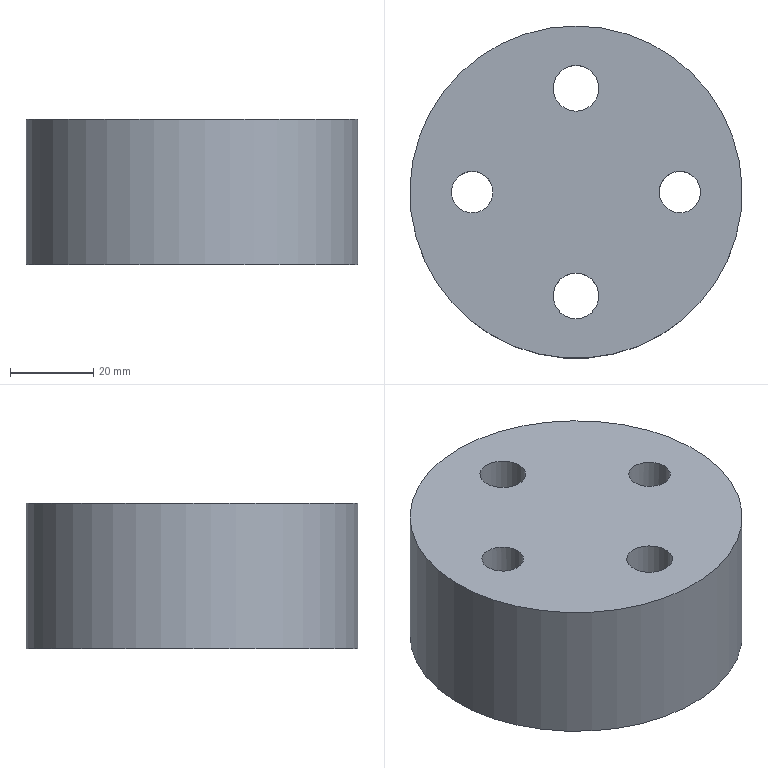Part | NX | features solid 2 | 1 solid | 14 faces | box 80 x 80 x 35 mm | volume 136848 mm3 | cylinder 8 | plane 5 | cone 1 | commonest cylinder face diameters 10 x2 11 x2 17 x2 5 x1 80 x1
STEP:
#1=CARTESIAN_POINT('',(1230.,-115.,-10.));
#2=VERTEX_POINT('',#1);
#3=CARTESIAN_POINT('',(1230.,-155.,-10.));
#4=DIRECTION('',(0.,0.,1.));
#5=DIRECTION('',(0.,1.,0.));
#6=AXIS2_PLACEMENT_3D('',#3,#4,#5);
#7=CIRCLE('',#6,40.);
#8=EDGE_CURVE('',#2,#2,#7,.T.);
#9=ORIENTED_EDGE('',*,*,#8,.F.);
#10=EDGE_LOOP('',(#9));
#11=FACE_BOUND('',#10,.T.);
#12=CARTESIAN_POINT('',(1230.,-121.225,-10.));
#13=VERTEX_POINT('',#12);
#14=CARTESIAN_POINT('',(1230.,-155.,-10.));
#15=DIRECTION('',(0.,0.,1.));
#16=DIRECTION('',(0.,1.,0.));
#17=AXIS2_PLACEMENT_3D('',#14,#15,#16);
#18=CIRCLE('',#17,33.775);
#19=EDGE_CURVE('',#13,#13,#18,.F.);
#20=ORIENTED_EDGE('',*,*,#19,.F.);
#21=EDGE_LOOP('',(#20));
#22=FACE_BOUND('',#21,.T.);
#23=CARTESIAN_POINT('',(1230.,-155.,-10.));
#24=DIRECTION('',(0.,0.,-1.));
#25=DIRECTION('',(0.,1.,0.));
#26=AXIS2_PLACEMENT_3D('',#23,#24,#25);
#27=PLANE('',#26);
#28=ADVANCED_FACE('',(#11,#22),#27,.T.);
#29=CARTESIAN_POINT('',(1230.,-171.5,15.));
#30=VERTEX_POINT('',#29);
#31=CARTESIAN_POINT('',(1230.,-180.,15.));
#32=DIRECTION('',(0.,0.,1.));
#33=DIRECTION('',(0.,1.,0.));
#34=AXIS2_PLACEMENT_3D('',#31,#32,#33);
#35=CIRCLE('',#34,8.5);
#36=EDGE_CURVE('',#30,#30,#35,.T.);
#37=ORIENTED_EDGE('',*,*,#36,.T.);
#38=EDGE_LOOP('',(#37));
#39=FACE_BOUND('',#38,.T.);
#40=CARTESIAN_POINT('',(1232.133,-171.772,-0.2613));
#41=VERTEX_POINT('',#40);
#42=CARTESIAN_POINT('',(1235.334,-173.116,-1.388));
#43=CARTESIAN_POINT('',(1232.24,-171.537,-0.06708));
#44=CARTESIAN_POINT('',(1228.503,-171.368,0.0881));
#45=CARTESIAN_POINT('',(1225.219,-172.711,-1.068));
#46=CARTESIAN_POINT('',(1222.909,-174.976,-2.736));
#47=CARTESIAN_POINT('',(1221.135,-178.794,-5.162));
#48=CARTESIAN_POINT('',(1221.604,-183.266,-7.482));
#49=CARTESIAN_POINT('',(1224.537,-186.821,-9.112));
#50=CARTESIAN_POINT('',(1227.755,-188.463,-9.826));
#51=CARTESIAN_POINT('',(1231.445,-188.641,-9.902));
#52=CARTESIAN_POINT('',(1235.993,-186.822,-9.118));
#53=CARTESIAN_POINT('',(1238.545,-182.748,-7.247));
#54=CARTESIAN_POINT('',(1238.556,-178.475,-4.925));
#55=CARTESIAN_POINT('',(1237.446,-175.519,-3.102));
#56=CARTESIAN_POINT('',(1235.334,-173.116,-1.388));
#57=CARTESIAN_POINT('',(1232.24,-171.537,-0.06708));
#58=CARTESIAN_POINT('',(1228.503,-171.368,0.0881));
#59=B_SPLINE_CURVE_WITH_KNOTS('',3,(#42,#43,#44,#45,#46,#47,#48,#49,#50,#51,#52,#53,#54,#55,#56,#57,#58),.UNSPECIFIED.,.T.,.F.,(1,1,1,1,1,1,1,1,1,1,1,1,1,1,1,1,1,1,1,1,1),(-0.01077,-0.007179,-0.00359,0.,0.00359,0.007179,0.01077,0.01436,0.02154,0.02513,0.02872,0.03231,0.0359,0.04307,0.04666,0.05025,0.05384,0.05743,0.06102,0.06461,0.0682),.UNSPECIFIED.);
#60=EDGE_CURVE('',#41,#41,#59,.T.);
#61=ORIENTED_EDGE('',*,*,#60,.F.);
#62=EDGE_LOOP('',(#61));
#63=FACE_BOUND('',#62,.T.);
#64=CARTESIAN_POINT('',(1230.,-180.,-10.));
#65=DIRECTION('',(0.,0.,1.));
#66=DIRECTION('',(0.,-1.,0.));
#67=AXIS2_PLACEMENT_3D('',#64,#65,#66);
#68=CYLINDRICAL_SURFACE('',#67,8.5);
#69=ADVANCED_FACE('',(#39,#63),#68,.F.);
#70=CARTESIAN_POINT('',(1230.,-121.5,15.));
#71=VERTEX_POINT('',#70);
#72=CARTESIAN_POINT('',(1230.,-130.,15.));
#73=DIRECTION('',(0.,0.,1.));
#74=DIRECTION('',(0.,1.,0.));
#75=AXIS2_PLACEMENT_3D('',#72,#73,#74);
#76=CIRCLE('',#75,8.5);
#77=EDGE_CURVE('',#71,#71,#76,.T.);
#78=ORIENTED_EDGE('',*,*,#77,.T.);
#79=EDGE_LOOP('',(#78));
#80=FACE_BOUND('',#79,.T.);
#81=CARTESIAN_POINT('',(1232.133,-138.228,-0.2613));
#82=VERTEX_POINT('',#81);
#83=CARTESIAN_POINT('',(1228.487,-138.633,0.08799));
#84=CARTESIAN_POINT('',(1232.248,-138.46,-0.06903));
#85=CARTESIAN_POINT('',(1235.319,-136.894,-1.38));
#86=CARTESIAN_POINT('',(1237.448,-134.481,-3.102));
#87=CARTESIAN_POINT('',(1238.554,-131.529,-4.923));
#88=CARTESIAN_POINT('',(1238.547,-127.268,-7.238));
#89=CARTESIAN_POINT('',(1236.016,-123.209,-9.105));
#90=CARTESIAN_POINT('',(1231.512,-121.372,-9.896));
#91=CARTESIAN_POINT('',(1227.809,-121.519,-9.834));
#92=CARTESIAN_POINT('',(1224.566,-123.154,-9.123));
#93=CARTESIAN_POINT('',(1222.35,-125.818,-7.901));
#94=CARTESIAN_POINT('',(1221.36,-128.972,-6.327));
#95=CARTESIAN_POINT('',(1221.58,-132.155,-4.557));
#96=CARTESIAN_POINT('',(1222.906,-135.021,-2.739));
#97=CARTESIAN_POINT('',(1225.207,-137.28,-1.075));
#98=CARTESIAN_POINT('',(1228.487,-138.633,0.08799));
#99=CARTESIAN_POINT('',(1232.248,-138.46,-0.06903));
#100=CARTESIAN_POINT('',(1235.319,-136.894,-1.38));
#101=B_SPLINE_CURVE_WITH_KNOTS('',3,(#83,#84,#85,#86,#87,#88,#89,#90,#91,#92,#93,#94,#95,#96,#97,#98,#99,#100),.UNSPECIFIED.,.T.,.F.,(1,1,1,1,1,1,1,1,1,1,1,1,1,1,1,1,1,1,1,1,1,1),(-0.01073,-0.007156,-0.003578,0.,0.003578,0.007156,0.01073,0.01431,0.02147,0.02505,0.02862,0.0322,0.03578,0.03936,0.04294,0.04651,0.05009,0.05367,0.05725,0.06083,0.0644,0.06798),.UNSPECIFIED.);
#102=EDGE_CURVE('',#82,#82,#101,.T.);
#103=ORIENTED_EDGE('',*,*,#102,.F.);
#104=EDGE_LOOP('',(#103));
#105=FACE_BOUND('',#104,.T.);
#106=CARTESIAN_POINT('',(1230.,-130.,-10.));
#107=DIRECTION('',(0.,0.,1.));
#108=DIRECTION('',(0.,-1.,0.));
#109=AXIS2_PLACEMENT_3D('',#106,#107,#108);
#110=CYLINDRICAL_SURFACE('',#109,8.5);
#111=ADVANCED_FACE('',(#80,#105),#110,.F.);
#112=CARTESIAN_POINT('',(1255.,-150.,25.));
#113=VERTEX_POINT('',#112);
#114=CARTESIAN_POINT('',(1255.,-155.,25.));
#115=DIRECTION('',(0.,0.,1.));
#116=DIRECTION('',(0.,1.,0.));
#117=AXIS2_PLACEMENT_3D('',#114,#115,#116);
#118=CIRCLE('',#117,5.);
#119=EDGE_CURVE('',#113,#113,#118,.T.);
#120=ORIENTED_EDGE('',*,*,#119,.T.);
#121=EDGE_LOOP('',(#120));
#122=FACE_BOUND('',#121,.T.);
#123=CARTESIAN_POINT('',(1255.794,-159.937,-5.662));
#124=VERTEX_POINT('',#123);
#125=CARTESIAN_POINT('',(1252.677,-159.733,-3.871));
#126=CARTESIAN_POINT('',(1255.826,-160.41,-5.731));
#127=CARTESIAN_POINT('',(1258.815,-158.719,-7.248));
#128=CARTESIAN_POINT('',(1260.021,-156.153,-7.831));
#129=CARTESIAN_POINT('',(1260.063,-153.241,-7.851));
#130=CARTESIAN_POINT('',(1257.855,-150.263,-6.789));
#131=CARTESIAN_POINT('',(1254.604,-149.757,-5.026));
#132=CARTESIAN_POINT('',(1252.298,-150.657,-3.614));
#133=CARTESIAN_POINT('',(1250.872,-151.956,-2.67));
#134=CARTESIAN_POINT('',(1249.984,-153.829,-2.036));
#135=CARTESIAN_POINT('',(1249.95,-156.028,-2.012));
#136=CARTESIAN_POINT('',(1250.8,-157.948,-2.619));
#137=CARTESIAN_POINT('',(1252.677,-159.733,-3.871));
#138=CARTESIAN_POINT('',(1255.826,-160.41,-5.731));
#139=CARTESIAN_POINT('',(1258.815,-158.719,-7.248));
#140=B_SPLINE_CURVE_WITH_KNOTS('',3,(#125,#126,#127,#128,#129,#130,#131,#132,#133,#134,#135,#136,#137,#138,#139),.UNSPECIFIED.,.T.,.F.,(1,1,1,1,1,1,1,1,1,1,1,1,1,1,1,1,1,1,1),(-0.008415,-0.006311,-0.004207,0.,0.004207,0.006311,0.008415,0.01262,0.01683,0.01893,0.02104,0.02314,0.02524,0.02735,0.02945,0.03366,0.03787,0.03997,0.04207),.UNSPECIFIED.);
#141=EDGE_CURVE('',#124,#124,#140,.T.);
#142=ORIENTED_EDGE('',*,*,#141,.F.);
#143=EDGE_LOOP('',(#142));
#144=FACE_BOUND('',#143,.T.);
#145=CARTESIAN_POINT('',(1255.,-155.,-10.));
#146=DIRECTION('',(0.,0.,1.));
#147=DIRECTION('',(0.,-1.,0.));
#148=AXIS2_PLACEMENT_3D('',#145,#146,#147);
#149=CYLINDRICAL_SURFACE('',#148,5.);
#150=ADVANCED_FACE('',(#122,#144),#149,.F.);
#151=CARTESIAN_POINT('',(1205.,-150.,25.));
#152=VERTEX_POINT('',#151);
#153=CARTESIAN_POINT('',(1205.,-155.,25.));
#154=DIRECTION('',(0.,0.,1.));
#155=DIRECTION('',(0.,1.,0.));
#156=AXIS2_PLACEMENT_3D('',#153,#154,#155);
#157=CIRCLE('',#156,5.);
#158=EDGE_CURVE('',#152,#152,#157,.T.);
#159=ORIENTED_EDGE('',*,*,#158,.T.);
#160=EDGE_LOOP('',(#159));
#161=FACE_BOUND('',#160,.T.);
#162=CARTESIAN_POINT('',(1209.151,-157.787,-2.644));
#163=VERTEX_POINT('',#162);
#164=CARTESIAN_POINT('',(1207.856,-159.244,-3.515));
#165=CARTESIAN_POINT('',(1209.247,-157.882,-2.587));
#166=CARTESIAN_POINT('',(1210.064,-155.948,-2.001));
#167=CARTESIAN_POINT('',(1210.,-153.762,-2.048));
#168=CARTESIAN_POINT('',(1209.081,-151.891,-2.702));
#169=CARTESIAN_POINT('',(1207.155,-150.194,-3.975));
#170=CARTESIAN_POINT('',(1204.,-149.617,-5.825));
#171=CARTESIAN_POINT('',(1201.052,-151.418,-7.313));
#172=CARTESIAN_POINT('',(1199.938,-154.037,-7.851));
#173=CARTESIAN_POINT('',(1200.012,-156.963,-7.815));
#174=CARTESIAN_POINT('',(1202.318,-159.83,-6.702));
#175=CARTESIAN_POINT('',(1205.581,-160.226,-4.919));
#176=CARTESIAN_POINT('',(1207.856,-159.244,-3.515));
#177=CARTESIAN_POINT('',(1209.247,-157.882,-2.587));
#178=CARTESIAN_POINT('',(1210.064,-155.948,-2.001));
#179=B_SPLINE_CURVE_WITH_KNOTS('',3,(#164,#165,#166,#167,#168,#169,#170,#171,#172,#173,#174,#175,#176,#177,#178),.UNSPECIFIED.,.T.,.F.,(1,1,1,1,1,1,1,1,1,1,1,1,1,1,1,1,1,1,1),(-0.008441,-0.004221,-0.00211,0.,0.00211,0.004221,0.006331,0.008441,0.01266,0.01688,0.01899,0.0211,0.02532,0.02954,0.03165,0.03376,0.03588,0.03799,0.0401),.UNSPECIFIED.);
#180=EDGE_CURVE('',#163,#163,#179,.T.);
#181=ORIENTED_EDGE('',*,*,#180,.F.);
#182=EDGE_LOOP('',(#181));
#183=FACE_BOUND('',#182,.T.);
#184=CARTESIAN_POINT('',(1205.,-155.,-10.));
#185=DIRECTION('',(0.,0.,1.));
#186=DIRECTION('',(0.,-1.,0.));
#187=AXIS2_PLACEMENT_3D('',#184,#185,#186);
#188=CYLINDRICAL_SURFACE('',#187,5.);
#189=ADVANCED_FACE('',(#161,#183),#188,.F.);
#190=ORIENTED_EDGE('',*,*,#119,.F.);
#191=EDGE_LOOP('',(#190));
#192=FACE_BOUND('',#191,.T.);
#193=CARTESIAN_POINT('',(1230.,-174.5,25.));
#194=VERTEX_POINT('',#193);
#195=CARTESIAN_POINT('',(1230.,-180.,25.));
#196=DIRECTION('',(0.,0.,1.));
#197=DIRECTION('',(0.,1.,0.));
#198=AXIS2_PLACEMENT_3D('',#195,#196,#197);
#199=CIRCLE('',#198,5.5);
#200=EDGE_CURVE('',#194,#194,#199,.T.);
#201=ORIENTED_EDGE('',*,*,#200,.F.);
#202=EDGE_LOOP('',(#201));
#203=FACE_BOUND('',#202,.T.);
#204=CARTESIAN_POINT('',(1230.,-115.,25.));
#205=VERTEX_POINT('',#204);
#206=CARTESIAN_POINT('',(1230.,-155.,25.));
#207=DIRECTION('',(0.,0.,1.));
#208=DIRECTION('',(0.,1.,0.));
#209=AXIS2_PLACEMENT_3D('',#206,#207,#208);
#210=CIRCLE('',#209,40.);
#211=EDGE_CURVE('',#205,#205,#210,.T.);
#212=ORIENTED_EDGE('',*,*,#211,.T.);
#213=EDGE_LOOP('',(#212));
#214=FACE_BOUND('',#213,.T.);
#215=CARTESIAN_POINT('',(1230.,-124.5,25.));
#216=VERTEX_POINT('',#215);
#217=CARTESIAN_POINT('',(1230.,-130.,25.));
#218=DIRECTION('',(0.,0.,1.));
#219=DIRECTION('',(0.,1.,0.));
#220=AXIS2_PLACEMENT_3D('',#217,#218,#219);
#221=CIRCLE('',#220,5.5);
#222=EDGE_CURVE('',#216,#216,#221,.T.);
#223=ORIENTED_EDGE('',*,*,#222,.F.);
#224=EDGE_LOOP('',(#223));
#225=FACE_BOUND('',#224,.T.);
#226=ORIENTED_EDGE('',*,*,#158,.F.);
#227=EDGE_LOOP('',(#226));
#228=FACE_BOUND('',#227,.T.);
#229=CARTESIAN_POINT('',(1230.,-155.,25.));
#230=DIRECTION('',(0.,0.,-1.));
#231=DIRECTION('',(0.,1.,0.));
#232=AXIS2_PLACEMENT_3D('',#229,#230,#231);
#233=PLANE('',#232);
#234=ADVANCED_FACE('',(#192,#203,#214,#225,#228),#233,.F.);
#235=ORIENTED_EDGE('',*,*,#77,.F.);
#236=EDGE_LOOP('',(#235));
#237=FACE_BOUND('',#236,.T.);
#238=CARTESIAN_POINT('',(1230.,-124.5,15.));
#239=VERTEX_POINT('',#238);
#240=CARTESIAN_POINT('',(1230.,-130.,15.));
#241=DIRECTION('',(0.,0.,1.));
#242=DIRECTION('',(0.,1.,0.));
#243=AXIS2_PLACEMENT_3D('',#240,#241,#242);
#244=CIRCLE('',#243,5.5);
#245=EDGE_CURVE('',#239,#239,#244,.T.);
#246=ORIENTED_EDGE('',*,*,#245,.T.);
#247=EDGE_LOOP('',(#246));
#248=FACE_BOUND('',#247,.T.);
#249=CARTESIAN_POINT('',(1230.,-130.,15.));
#250=DIRECTION('',(0.,0.,-1.));
#251=DIRECTION('',(0.,1.,0.));
#252=AXIS2_PLACEMENT_3D('',#249,#250,#251);
#253=PLANE('',#252);
#254=ADVANCED_FACE('',(#237,#248),#253,.T.);
#255=ORIENTED_EDGE('',*,*,#36,.F.);
#256=EDGE_LOOP('',(#255));
#257=FACE_BOUND('',#256,.T.);
#258=CARTESIAN_POINT('',(1230.,-174.5,15.));
#259=VERTEX_POINT('',#258);
#260=CARTESIAN_POINT('',(1230.,-180.,15.));
#261=DIRECTION('',(0.,0.,1.));
#262=DIRECTION('',(0.,1.,0.));
#263=AXIS2_PLACEMENT_3D('',#260,#261,#262);
#264=CIRCLE('',#263,5.5);
#265=EDGE_CURVE('',#259,#259,#264,.T.);
#266=ORIENTED_EDGE('',*,*,#265,.T.);
#267=EDGE_LOOP('',(#266));
#268=FACE_BOUND('',#267,.T.);
#269=CARTESIAN_POINT('',(1230.,-180.,15.));
#270=DIRECTION('',(0.,0.,-1.));
#271=DIRECTION('',(0.,1.,0.));
#272=AXIS2_PLACEMENT_3D('',#269,#270,#271);
#273=PLANE('',#272);
#274=ADVANCED_FACE('',(#257,#268),#273,.T.);
#275=ORIENTED_EDGE('',*,*,#8,.T.);
#276=EDGE_LOOP('',(#275));
#277=FACE_BOUND('',#276,.T.);
#278=ORIENTED_EDGE('',*,*,#211,.F.);
#279=EDGE_LOOP('',(#278));
#280=FACE_BOUND('',#279,.T.);
#281=CARTESIAN_POINT('',(1230.,-155.,-10.));
#282=DIRECTION('',(0.,0.,1.));
#283=DIRECTION('',(0.,-1.,0.));
#284=AXIS2_PLACEMENT_3D('',#281,#282,#283);
#285=CYLINDRICAL_SURFACE('',#284,40.);
#286=ADVANCED_FACE('',(#277,#280),#285,.T.);
#287=ORIENTED_EDGE('',*,*,#265,.F.);
#288=EDGE_LOOP('',(#287));
#289=FACE_BOUND('',#288,.T.);
#290=ORIENTED_EDGE('',*,*,#200,.T.);
#291=EDGE_LOOP('',(#290));
#292=FACE_BOUND('',#291,.T.);
#293=CARTESIAN_POINT('',(1230.,-180.,15.));
#294=DIRECTION('',(0.,0.,1.));
#295=DIRECTION('',(0.,-1.,0.));
#296=AXIS2_PLACEMENT_3D('',#293,#294,#295);
#297=CYLINDRICAL_SURFACE('',#296,5.5);
#298=ADVANCED_FACE('',(#289,#292),#297,.F.);
#299=ORIENTED_EDGE('',*,*,#245,.F.);
#300=EDGE_LOOP('',(#299));
#301=FACE_BOUND('',#300,.T.);
#302=ORIENTED_EDGE('',*,*,#222,.T.);
#303=EDGE_LOOP('',(#302));
#304=FACE_BOUND('',#303,.T.);
#305=CARTESIAN_POINT('',(1230.,-130.,15.));
#306=DIRECTION('',(0.,0.,1.));
#307=DIRECTION('',(0.,-1.,0.));
#308=AXIS2_PLACEMENT_3D('',#305,#306,#307);
#309=CYLINDRICAL_SURFACE('',#308,5.5);
#310=ADVANCED_FACE('',(#301,#304),#309,.F.);
#311=ORIENTED_EDGE('',*,*,#19,.T.);
#312=EDGE_LOOP('',(#311));
#313=FACE_BOUND('',#312,.T.);
#314=ORIENTED_EDGE('',*,*,#60,.T.);
#315=EDGE_LOOP('',(#314));
#316=FACE_BOUND('',#315,.T.);
#317=ORIENTED_EDGE('',*,*,#102,.T.);
#318=EDGE_LOOP('',(#317));
#319=FACE_BOUND('',#318,.T.);
#320=ORIENTED_EDGE('',*,*,#141,.T.);
#321=EDGE_LOOP('',(#320));
#322=FACE_BOUND('',#321,.T.);
#323=ORIENTED_EDGE('',*,*,#180,.T.);
#324=EDGE_LOOP('',(#323));
#325=FACE_BOUND('',#324,.T.);
#326=CARTESIAN_POINT('',(1230.,-152.5,8.057));
#327=VERTEX_POINT('',#326);
#328=CARTESIAN_POINT('',(1230.,-155.,8.057));
#329=DIRECTION('',(0.,0.,1.));
#330=DIRECTION('',(0.,1.,0.));
#331=AXIS2_PLACEMENT_3D('',#328,#329,#330);
#332=CIRCLE('',#331,2.5);
#333=EDGE_CURVE('',#327,#327,#332,.F.);
#334=ORIENTED_EDGE('',*,*,#333,.F.);
#335=EDGE_LOOP('',(#334));
#336=FACE_BOUND('',#335,.T.);
#337=CARTESIAN_POINT('',(1230.,-155.,-13.594));
#338=DIRECTION('',(0.,0.,-1.));
#339=DIRECTION('',(0.,1.,0.));
#340=AXIS2_PLACEMENT_3D('',#337,#338,#339);
#341=CONICAL_SURFACE('',#340,40.,1.047);
#342=ADVANCED_FACE('',(#313,#316,#319,#322,#325,#336),#341,.F.);
#343=CARTESIAN_POINT('',(1230.,-157.5,10.));
#344=VERTEX_POINT('',#343);
#345=CARTESIAN_POINT('',(1230.,-155.,10.));
#346=DIRECTION('',(0.,0.,-1.));
#347=DIRECTION('',(0.,-1.,0.));
#348=AXIS2_PLACEMENT_3D('',#345,#346,#347);
#349=CIRCLE('',#348,2.5);
#350=EDGE_CURVE('',#344,#344,#349,.T.);
#351=ORIENTED_EDGE('',*,*,#350,.T.);
#352=EDGE_LOOP('',(#351));
#353=FACE_BOUND('',#352,.T.);
#354=CARTESIAN_POINT('',(1230.,-155.,10.));
#355=DIRECTION('',(0.,0.,1.));
#356=DIRECTION('',(0.,-1.,0.));
#357=AXIS2_PLACEMENT_3D('',#354,#355,#356);
#358=PLANE('',#357);
#359=ADVANCED_FACE('',(#353),#358,.F.);
#360=ORIENTED_EDGE('',*,*,#350,.F.);
#361=EDGE_LOOP('',(#360));
#362=FACE_BOUND('',#361,.T.);
#363=ORIENTED_EDGE('',*,*,#333,.T.);
#364=EDGE_LOOP('',(#363));
#365=FACE_BOUND('',#364,.T.);
#366=CARTESIAN_POINT('',(1230.,-155.,-10.));
#367=DIRECTION('',(0.,0.,1.));
#368=DIRECTION('',(0.,-1.,0.));
#369=AXIS2_PLACEMENT_3D('',#366,#367,#368);
#370=CYLINDRICAL_SURFACE('',#369,2.5);
#371=ADVANCED_FACE('',(#362,#365),#370,.F.);
#372=CLOSED_SHELL('',(#28,#69,#111,#150,#189,#234,#254,#274,#286,#298,#310,#342,#359,#371));
#373=MANIFOLD_SOLID_BREP('',#372);
#374=(LENGTH_UNIT()NAMED_UNIT(*)SI_UNIT(.MILLI.,.METRE.));
#375=UNCERTAINTY_MEASURE_WITH_UNIT(LENGTH_MEASURE(0.0508),#374,'','');
#376=(NAMED_UNIT(*)PLANE_ANGLE_UNIT()SI_UNIT($,.RADIAN.));
#377=(NAMED_UNIT(*)SI_UNIT($,.STERADIAN.)SOLID_ANGLE_UNIT());
#378=(GEOMETRIC_REPRESENTATION_CONTEXT(3)GLOBAL_UNCERTAINTY_ASSIGNED_CONTEXT((#375))GLOBAL_UNIT_ASSIGNED_CONTEXT((#374,#376,#377))REPRESENTATION_CONTEXT('',''));
#379=ADVANCED_BREP_SHAPE_REPRESENTATION('',(#373),#378);